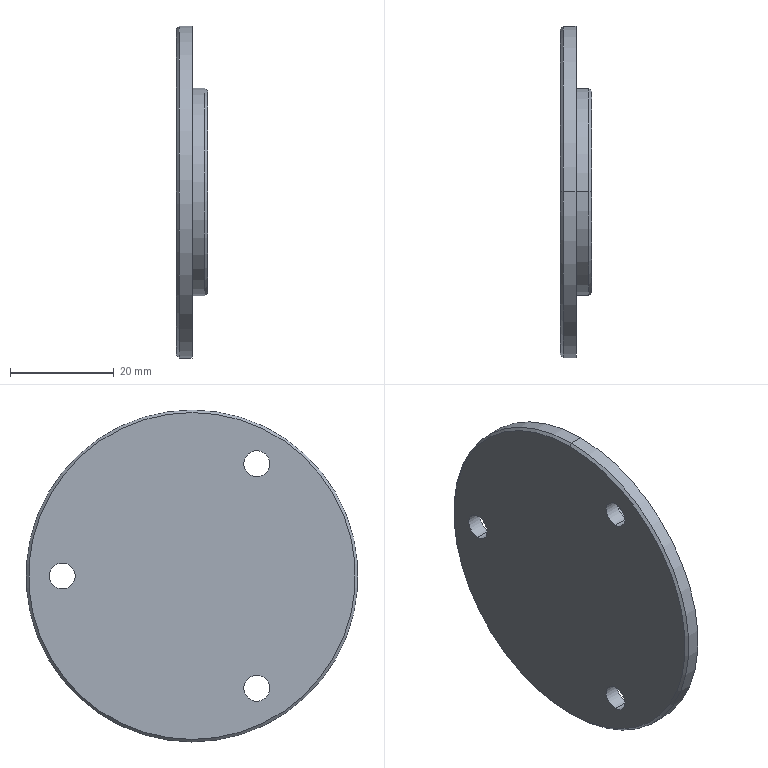Part | SolidWorks | features ICE 3, Chamfer 1, Extrusion 1 | 1 solid | 20 faces | box 6 x 64 x 64 mm | volume 11842 mm3 | cylinder 12 | cone 4 | plane 4 | commonest cylinder face diameters 5 x6 34 x2 40 x2 64 x2
STEP:
#1=CARTESIAN_POINT('',(0.,0.,31.5));
#2=VERTEX_POINT('',#1);
#3=CARTESIAN_POINT('',(0.,0.,-31.5));
#4=VERTEX_POINT('',#3);
#5=CARTESIAN_POINT('',(0.,0.,0.));
#6=DIRECTION('',(-1.,0.,0.));
#7=DIRECTION('',(0.,0.,-1.));
#8=AXIS2_PLACEMENT_3D('',#5,#6,#7);
#9=CIRCLE('',#8,31.5);
#10=EDGE_CURVE('',#2,#4,#9,.T.);
#11=ORIENTED_EDGE('',*,*,#10,.F.);
#12=CARTESIAN_POINT('',(0.5,0.,32.));
#13=VERTEX_POINT('',#12);
#14=CARTESIAN_POINT('',(0.5,0.,32.));
#15=DIRECTION('',(0.7071,0.,0.7071));
#16=VECTOR('',#15,1000.);
#17=LINE('',#14,#16);
#18=EDGE_CURVE('',#2,#13,#17,.T.);
#19=ORIENTED_EDGE('',*,*,#18,.T.);
#20=CARTESIAN_POINT('',(0.5,0.,-32.));
#21=VERTEX_POINT('',#20);
#22=CARTESIAN_POINT('',(0.5,0.,0.));
#23=DIRECTION('',(1.,0.,0.));
#24=DIRECTION('',(0.,0.,-1.));
#25=AXIS2_PLACEMENT_3D('',#22,#23,#24);
#26=CIRCLE('',#25,32.);
#27=EDGE_CURVE('',#21,#13,#26,.T.);
#28=ORIENTED_EDGE('',*,*,#27,.F.);
#29=CARTESIAN_POINT('',(0.5,0.,-32.));
#30=DIRECTION('',(0.7071,0.,-0.7071));
#31=VECTOR('',#30,1000.);
#32=LINE('',#29,#31);
#33=EDGE_CURVE('',#4,#21,#32,.T.);
#34=ORIENTED_EDGE('',*,*,#33,.F.);
#35=EDGE_LOOP('',(#11,#19,#28,#34));
#36=FACE_OUTER_BOUND('',#35,.T.);
#37=CARTESIAN_POINT('',(0.5,0.,0.));
#38=DIRECTION('',(1.,0.,0.));
#39=DIRECTION('',(0.,0.,-1.));
#40=AXIS2_PLACEMENT_3D('',#37,#38,#39);
#41=CONICAL_SURFACE('',#40,32.,0.7854);
#42=ADVANCED_FACE('',(#36),#41,.T.);
#43=CARTESIAN_POINT('',(6.,0.,-19.5));
#44=VERTEX_POINT('',#43);
#45=CARTESIAN_POINT('',(6.,0.,19.5));
#46=VERTEX_POINT('',#45);
#47=CARTESIAN_POINT('',(6.,0.,0.));
#48=DIRECTION('',(1.,0.,0.));
#49=DIRECTION('',(0.,0.,-1.));
#50=AXIS2_PLACEMENT_3D('',#47,#48,#49);
#51=CIRCLE('',#50,19.5);
#52=EDGE_CURVE('',#44,#46,#51,.T.);
#53=ORIENTED_EDGE('',*,*,#52,.F.);
#54=CARTESIAN_POINT('',(5.5,0.,-20.));
#55=VERTEX_POINT('',#54);
#56=CARTESIAN_POINT('',(6.,0.,-19.5));
#57=DIRECTION('',(-0.7071,0.,-0.7071));
#58=VECTOR('',#57,1000.);
#59=LINE('',#56,#58);
#60=EDGE_CURVE('',#44,#55,#59,.T.);
#61=ORIENTED_EDGE('',*,*,#60,.T.);
#62=CARTESIAN_POINT('',(5.5,0.,20.));
#63=VERTEX_POINT('',#62);
#64=CARTESIAN_POINT('',(5.5,0.,0.));
#65=DIRECTION('',(-1.,0.,0.));
#66=DIRECTION('',(0.,0.,-1.));
#67=AXIS2_PLACEMENT_3D('',#64,#65,#66);
#68=CIRCLE('',#67,20.);
#69=EDGE_CURVE('',#63,#55,#68,.T.);
#70=ORIENTED_EDGE('',*,*,#69,.F.);
#71=CARTESIAN_POINT('',(6.,0.,19.5));
#72=DIRECTION('',(-0.7071,0.,0.7071));
#73=VECTOR('',#72,1000.);
#74=LINE('',#71,#73);
#75=EDGE_CURVE('',#46,#63,#74,.T.);
#76=ORIENTED_EDGE('',*,*,#75,.F.);
#77=EDGE_LOOP('',(#53,#61,#70,#76));
#78=FACE_OUTER_BOUND('',#77,.T.);
#79=CARTESIAN_POINT('',(6.,0.,0.));
#80=DIRECTION('',(-1.,0.,0.));
#81=DIRECTION('',(0.,0.,1.));
#82=AXIS2_PLACEMENT_3D('',#79,#80,#81);
#83=CONICAL_SURFACE('',#82,19.5,0.7854);
#84=ADVANCED_FACE('',(#78),#83,.T.);
#85=CARTESIAN_POINT('',(3.,25.,2.5));
#86=VERTEX_POINT('',#85);
#87=CARTESIAN_POINT('',(3.,25.,-2.5));
#88=VERTEX_POINT('',#87);
#89=CARTESIAN_POINT('',(3.,25.,0.));
#90=DIRECTION('',(1.,0.,0.));
#91=DIRECTION('',(0.,0.,-1.));
#92=AXIS2_PLACEMENT_3D('',#89,#90,#91);
#93=CIRCLE('',#92,2.5);
#94=EDGE_CURVE('',#86,#88,#93,.T.);
#95=ORIENTED_EDGE('',*,*,#94,.T.);
#96=CARTESIAN_POINT('',(0.,25.,-2.5));
#97=VERTEX_POINT('',#96);
#98=CARTESIAN_POINT('',(36.5,25.,-2.5));
#99=DIRECTION('',(-1.,0.,0.));
#100=VECTOR('',#99,1000.);
#101=LINE('',#98,#100);
#102=EDGE_CURVE('',#88,#97,#101,.T.);
#103=ORIENTED_EDGE('',*,*,#102,.T.);
#104=CARTESIAN_POINT('',(0.,25.,2.5));
#105=VERTEX_POINT('',#104);
#106=CARTESIAN_POINT('',(0.,25.,0.));
#107=DIRECTION('',(-1.,0.,0.));
#108=DIRECTION('',(0.,0.,1.));
#109=AXIS2_PLACEMENT_3D('',#106,#107,#108);
#110=CIRCLE('',#109,2.5);
#111=EDGE_CURVE('',#97,#105,#110,.T.);
#112=ORIENTED_EDGE('',*,*,#111,.T.);
#113=CARTESIAN_POINT('',(36.5,25.,2.5));
#114=DIRECTION('',(-1.,0.,0.));
#115=VECTOR('',#114,1000.);
#116=LINE('',#113,#115);
#117=EDGE_CURVE('',#86,#105,#116,.T.);
#118=ORIENTED_EDGE('',*,*,#117,.F.);
#119=EDGE_LOOP('',(#95,#103,#112,#118));
#120=FACE_OUTER_BOUND('',#119,.T.);
#121=CARTESIAN_POINT('',(36.5,25.,0.));
#122=DIRECTION('',(-1.,0.,0.));
#123=DIRECTION('',(0.,0.,1.));
#124=AXIS2_PLACEMENT_3D('',#121,#122,#123);
#125=CYLINDRICAL_SURFACE('',#124,2.5);
#126=ADVANCED_FACE('',(#120),#125,.F.);
#127=CARTESIAN_POINT('',(3.,-12.5,24.151));
#128=VERTEX_POINT('',#127);
#129=CARTESIAN_POINT('',(3.,-12.5,19.151));
#130=VERTEX_POINT('',#129);
#131=CARTESIAN_POINT('',(3.,-12.5,21.651));
#132=DIRECTION('',(1.,0.,0.));
#133=DIRECTION('',(0.,0.,-1.));
#134=AXIS2_PLACEMENT_3D('',#131,#132,#133);
#135=CIRCLE('',#134,2.5);
#136=EDGE_CURVE('',#128,#130,#135,.T.);
#137=ORIENTED_EDGE('',*,*,#136,.T.);
#138=CARTESIAN_POINT('',(0.,-12.5,19.151));
#139=VERTEX_POINT('',#138);
#140=CARTESIAN_POINT('',(36.5,-12.5,19.151));
#141=DIRECTION('',(-1.,0.,0.));
#142=VECTOR('',#141,1000.);
#143=LINE('',#140,#142);
#144=EDGE_CURVE('',#130,#139,#143,.T.);
#145=ORIENTED_EDGE('',*,*,#144,.T.);
#146=CARTESIAN_POINT('',(0.,-12.5,24.151));
#147=VERTEX_POINT('',#146);
#148=CARTESIAN_POINT('',(0.,-12.5,21.651));
#149=DIRECTION('',(-1.,0.,0.));
#150=DIRECTION('',(0.,0.,1.));
#151=AXIS2_PLACEMENT_3D('',#148,#149,#150);
#152=CIRCLE('',#151,2.5);
#153=EDGE_CURVE('',#139,#147,#152,.T.);
#154=ORIENTED_EDGE('',*,*,#153,.T.);
#155=CARTESIAN_POINT('',(36.5,-12.5,24.151));
#156=DIRECTION('',(-1.,0.,0.));
#157=VECTOR('',#156,1000.);
#158=LINE('',#155,#157);
#159=EDGE_CURVE('',#128,#147,#158,.T.);
#160=ORIENTED_EDGE('',*,*,#159,.F.);
#161=EDGE_LOOP('',(#137,#145,#154,#160));
#162=FACE_OUTER_BOUND('',#161,.T.);
#163=CARTESIAN_POINT('',(36.5,-12.5,21.651));
#164=DIRECTION('',(-1.,0.,0.));
#165=DIRECTION('',(0.,0.,1.));
#166=AXIS2_PLACEMENT_3D('',#163,#164,#165);
#167=CYLINDRICAL_SURFACE('',#166,2.5);
#168=ADVANCED_FACE('',(#162),#167,.F.);
#169=CARTESIAN_POINT('',(3.,-12.5,-19.151));
#170=VERTEX_POINT('',#169);
#171=CARTESIAN_POINT('',(3.,-12.5,-24.151));
#172=VERTEX_POINT('',#171);
#173=CARTESIAN_POINT('',(3.,-12.5,-21.651));
#174=DIRECTION('',(1.,0.,0.));
#175=DIRECTION('',(0.,0.,-1.));
#176=AXIS2_PLACEMENT_3D('',#173,#174,#175);
#177=CIRCLE('',#176,2.5);
#178=EDGE_CURVE('',#170,#172,#177,.T.);
#179=ORIENTED_EDGE('',*,*,#178,.T.);
#180=CARTESIAN_POINT('',(0.,-12.5,-24.151));
#181=VERTEX_POINT('',#180);
#182=CARTESIAN_POINT('',(36.5,-12.5,-24.151));
#183=DIRECTION('',(-1.,0.,0.));
#184=VECTOR('',#183,1000.);
#185=LINE('',#182,#184);
#186=EDGE_CURVE('',#172,#181,#185,.T.);
#187=ORIENTED_EDGE('',*,*,#186,.T.);
#188=CARTESIAN_POINT('',(0.,-12.5,-19.151));
#189=VERTEX_POINT('',#188);
#190=CARTESIAN_POINT('',(0.,-12.5,-21.651));
#191=DIRECTION('',(-1.,0.,0.));
#192=DIRECTION('',(0.,0.,1.));
#193=AXIS2_PLACEMENT_3D('',#190,#191,#192);
#194=CIRCLE('',#193,2.5);
#195=EDGE_CURVE('',#181,#189,#194,.T.);
#196=ORIENTED_EDGE('',*,*,#195,.T.);
#197=CARTESIAN_POINT('',(36.5,-12.5,-19.151));
#198=DIRECTION('',(-1.,0.,0.));
#199=VECTOR('',#198,1000.);
#200=LINE('',#197,#199);
#201=EDGE_CURVE('',#170,#189,#200,.T.);
#202=ORIENTED_EDGE('',*,*,#201,.F.);
#203=EDGE_LOOP('',(#179,#187,#196,#202));
#204=FACE_OUTER_BOUND('',#203,.T.);
#205=CARTESIAN_POINT('',(36.5,-12.5,-21.651));
#206=DIRECTION('',(-1.,0.,0.));
#207=DIRECTION('',(0.,0.,1.));
#208=AXIS2_PLACEMENT_3D('',#205,#206,#207);
#209=CYLINDRICAL_SURFACE('',#208,2.5);
#210=ADVANCED_FACE('',(#204),#209,.F.);
#211=CARTESIAN_POINT('',(4.5,0.,17.));
#212=VERTEX_POINT('',#211);
#213=CARTESIAN_POINT('',(4.5,0.,-17.));
#214=VERTEX_POINT('',#213);
#215=CARTESIAN_POINT('',(4.5,0.,0.));
#216=DIRECTION('',(1.,0.,0.));
#217=DIRECTION('',(0.,0.,-1.));
#218=AXIS2_PLACEMENT_3D('',#215,#216,#217);
#219=CIRCLE('',#218,17.);
#220=EDGE_CURVE('',#212,#214,#219,.T.);
#221=ORIENTED_EDGE('',*,*,#220,.F.);
#222=CARTESIAN_POINT('',(6.,0.,17.));
#223=VERTEX_POINT('',#222);
#224=CARTESIAN_POINT('',(4.5,0.,17.));
#225=DIRECTION('',(1.,0.,0.));
#226=VECTOR('',#225,1000.);
#227=LINE('',#224,#226);
#228=EDGE_CURVE('',#212,#223,#227,.T.);
#229=ORIENTED_EDGE('',*,*,#228,.T.);
#230=CARTESIAN_POINT('',(6.,0.,-17.));
#231=VERTEX_POINT('',#230);
#232=CARTESIAN_POINT('',(6.,0.,0.));
#233=DIRECTION('',(1.,0.,0.));
#234=DIRECTION('',(0.,0.,-1.));
#235=AXIS2_PLACEMENT_3D('',#232,#233,#234);
#236=CIRCLE('',#235,17.);
#237=EDGE_CURVE('',#223,#231,#236,.T.);
#238=ORIENTED_EDGE('',*,*,#237,.T.);
#239=CARTESIAN_POINT('',(4.5,0.,-17.));
#240=DIRECTION('',(1.,0.,0.));
#241=VECTOR('',#240,1000.);
#242=LINE('',#239,#241);
#243=EDGE_CURVE('',#214,#231,#242,.T.);
#244=ORIENTED_EDGE('',*,*,#243,.F.);
#245=EDGE_LOOP('',(#221,#229,#238,#244));
#246=FACE_OUTER_BOUND('',#245,.T.);
#247=CARTESIAN_POINT('',(4.5,0.,0.));
#248=DIRECTION('',(1.,0.,0.));
#249=DIRECTION('',(0.,0.,-1.));
#250=AXIS2_PLACEMENT_3D('',#247,#248,#249);
#251=CYLINDRICAL_SURFACE('',#250,17.);
#252=ADVANCED_FACE('',(#246),#251,.F.);
#253=ORIENTED_EDGE('',*,*,#69,.T.);
#254=CARTESIAN_POINT('',(3.,0.,-20.));
#255=VERTEX_POINT('',#254);
#256=CARTESIAN_POINT('',(6.,0.,-20.));
#257=DIRECTION('',(-1.,0.,0.));
#258=VECTOR('',#257,1000.);
#259=LINE('',#256,#258);
#260=EDGE_CURVE('',#55,#255,#259,.T.);
#261=ORIENTED_EDGE('',*,*,#260,.T.);
#262=CARTESIAN_POINT('',(3.,0.,20.));
#263=VERTEX_POINT('',#262);
#264=CARTESIAN_POINT('',(3.,0.,0.));
#265=DIRECTION('',(1.,0.,0.));
#266=DIRECTION('',(0.,0.,-1.));
#267=AXIS2_PLACEMENT_3D('',#264,#265,#266);
#268=CIRCLE('',#267,20.);
#269=EDGE_CURVE('',#255,#263,#268,.T.);
#270=ORIENTED_EDGE('',*,*,#269,.T.);
#271=CARTESIAN_POINT('',(6.,0.,20.));
#272=DIRECTION('',(-1.,0.,0.));
#273=VECTOR('',#272,1000.);
#274=LINE('',#271,#273);
#275=EDGE_CURVE('',#63,#263,#274,.T.);
#276=ORIENTED_EDGE('',*,*,#275,.F.);
#277=EDGE_LOOP('',(#253,#261,#270,#276));
#278=FACE_OUTER_BOUND('',#277,.T.);
#279=CARTESIAN_POINT('',(6.,0.,0.));
#280=DIRECTION('',(-1.,0.,0.));
#281=DIRECTION('',(0.,0.,1.));
#282=AXIS2_PLACEMENT_3D('',#279,#280,#281);
#283=CYLINDRICAL_SURFACE('',#282,20.);
#284=ADVANCED_FACE('',(#278),#283,.T.);
#285=CARTESIAN_POINT('',(3.,0.,-32.));
#286=VERTEX_POINT('',#285);
#287=CARTESIAN_POINT('',(3.,0.,32.));
#288=VERTEX_POINT('',#287);
#289=CARTESIAN_POINT('',(3.,0.,0.));
#290=DIRECTION('',(1.,0.,0.));
#291=DIRECTION('',(0.,0.,-1.));
#292=AXIS2_PLACEMENT_3D('',#289,#290,#291);
#293=CIRCLE('',#292,32.);
#294=EDGE_CURVE('',#286,#288,#293,.T.);
#295=ORIENTED_EDGE('',*,*,#294,.F.);
#296=CARTESIAN_POINT('',(3.,0.,-32.));
#297=DIRECTION('',(-1.,0.,0.));
#298=VECTOR('',#297,1000.);
#299=LINE('',#296,#298);
#300=EDGE_CURVE('',#286,#21,#299,.T.);
#301=ORIENTED_EDGE('',*,*,#300,.T.);
#302=ORIENTED_EDGE('',*,*,#27,.T.);
#303=CARTESIAN_POINT('',(3.,0.,32.));
#304=DIRECTION('',(-1.,0.,0.));
#305=VECTOR('',#304,1000.);
#306=LINE('',#303,#305);
#307=EDGE_CURVE('',#288,#13,#306,.T.);
#308=ORIENTED_EDGE('',*,*,#307,.F.);
#309=EDGE_LOOP('',(#295,#301,#302,#308));
#310=FACE_OUTER_BOUND('',#309,.T.);
#311=CARTESIAN_POINT('',(3.,0.,0.));
#312=DIRECTION('',(-1.,0.,0.));
#313=DIRECTION('',(0.,0.,1.));
#314=AXIS2_PLACEMENT_3D('',#311,#312,#313);
#315=CYLINDRICAL_SURFACE('',#314,32.);
#316=ADVANCED_FACE('',(#310),#315,.T.);
#317=ORIENTED_EDGE('',*,*,#300,.F.);
#318=CARTESIAN_POINT('',(3.,0.,0.));
#319=DIRECTION('',(1.,0.,0.));
#320=DIRECTION('',(0.,0.,-1.));
#321=AXIS2_PLACEMENT_3D('',#318,#319,#320);
#322=CIRCLE('',#321,32.);
#323=EDGE_CURVE('',#288,#286,#322,.T.);
#324=ORIENTED_EDGE('',*,*,#323,.F.);
#325=ORIENTED_EDGE('',*,*,#307,.T.);
#326=CARTESIAN_POINT('',(0.5,0.,0.));
#327=DIRECTION('',(1.,0.,0.));
#328=DIRECTION('',(0.,0.,-1.));
#329=AXIS2_PLACEMENT_3D('',#326,#327,#328);
#330=CIRCLE('',#329,32.);
#331=EDGE_CURVE('',#13,#21,#330,.T.);
#332=ORIENTED_EDGE('',*,*,#331,.T.);
#333=EDGE_LOOP('',(#317,#324,#325,#332));
#334=FACE_OUTER_BOUND('',#333,.T.);
#335=CARTESIAN_POINT('',(3.,0.,0.));
#336=DIRECTION('',(-1.,0.,0.));
#337=DIRECTION('',(0.,0.,1.));
#338=AXIS2_PLACEMENT_3D('',#335,#336,#337);
#339=CYLINDRICAL_SURFACE('',#338,32.);
#340=ADVANCED_FACE('',(#334),#339,.T.);
#341=ORIENTED_EDGE('',*,*,#94,.F.);
#342=CARTESIAN_POINT('',(3.,25.,0.));
#343=DIRECTION('',(1.,0.,0.));
#344=DIRECTION('',(0.,0.,-1.));
#345=AXIS2_PLACEMENT_3D('',#342,#343,#344);
#346=CIRCLE('',#345,2.5);
#347=EDGE_CURVE('',#88,#86,#346,.T.);
#348=ORIENTED_EDGE('',*,*,#347,.F.);
#349=EDGE_LOOP('',(#341,#348));
#350=FACE_BOUND('',#349,.T.);
#351=ORIENTED_EDGE('',*,*,#136,.F.);
#352=CARTESIAN_POINT('',(3.,-12.5,21.651));
#353=DIRECTION('',(1.,0.,0.));
#354=DIRECTION('',(0.,0.,-1.));
#355=AXIS2_PLACEMENT_3D('',#352,#353,#354);
#356=CIRCLE('',#355,2.5);
#357=EDGE_CURVE('',#130,#128,#356,.T.);
#358=ORIENTED_EDGE('',*,*,#357,.F.);
#359=EDGE_LOOP('',(#351,#358));
#360=FACE_BOUND('',#359,.T.);
#361=ORIENTED_EDGE('',*,*,#178,.F.);
#362=CARTESIAN_POINT('',(3.,-12.5,-21.651));
#363=DIRECTION('',(1.,0.,0.));
#364=DIRECTION('',(0.,0.,-1.));
#365=AXIS2_PLACEMENT_3D('',#362,#363,#364);
#366=CIRCLE('',#365,2.5);
#367=EDGE_CURVE('',#172,#170,#366,.T.);
#368=ORIENTED_EDGE('',*,*,#367,.F.);
#369=EDGE_LOOP('',(#361,#368));
#370=FACE_BOUND('',#369,.T.);
#371=CARTESIAN_POINT('',(3.,0.,0.));
#372=DIRECTION('',(1.,0.,0.));
#373=DIRECTION('',(0.,0.,-1.));
#374=AXIS2_PLACEMENT_3D('',#371,#372,#373);
#375=CIRCLE('',#374,20.);
#376=EDGE_CURVE('',#263,#255,#375,.T.);
#377=ORIENTED_EDGE('',*,*,#376,.F.);
#378=ORIENTED_EDGE('',*,*,#269,.F.);
#379=EDGE_LOOP('',(#377,#378));
#380=FACE_BOUND('',#379,.T.);
#381=ORIENTED_EDGE('',*,*,#323,.T.);
#382=ORIENTED_EDGE('',*,*,#294,.T.);
#383=EDGE_LOOP('',(#381,#382));
#384=FACE_OUTER_BOUND('',#383,.T.);
#385=CARTESIAN_POINT('',(3.,0.,0.));
#386=DIRECTION('',(1.,0.,0.));
#387=DIRECTION('',(0.,0.,-1.));
#388=AXIS2_PLACEMENT_3D('',#385,#386,#387);
#389=PLANE('',#388);
#390=ADVANCED_FACE('',(#350,#360,#370,#380,#384),#389,.T.);
#391=CARTESIAN_POINT('',(0.,0.,0.));
#392=DIRECTION('',(-1.,0.,0.));
#393=DIRECTION('',(0.,0.,-1.));
#394=AXIS2_PLACEMENT_3D('',#391,#392,#393);
#395=CIRCLE('',#394,31.5);
#396=EDGE_CURVE('',#4,#2,#395,.T.);
#397=ORIENTED_EDGE('',*,*,#396,.T.);
#398=ORIENTED_EDGE('',*,*,#10,.T.);
#399=EDGE_LOOP('',(#397,#398));
#400=FACE_OUTER_BOUND('',#399,.T.);
#401=CARTESIAN_POINT('',(0.,25.,0.));
#402=DIRECTION('',(-1.,0.,0.));
#403=DIRECTION('',(0.,0.,1.));
#404=AXIS2_PLACEMENT_3D('',#401,#402,#403);
#405=CIRCLE('',#404,2.5);
#406=EDGE_CURVE('',#105,#97,#405,.T.);
#407=ORIENTED_EDGE('',*,*,#406,.F.);
#408=ORIENTED_EDGE('',*,*,#111,.F.);
#409=EDGE_LOOP('',(#407,#408));
#410=FACE_BOUND('',#409,.T.);
#411=CARTESIAN_POINT('',(0.,-12.5,21.651));
#412=DIRECTION('',(-1.,0.,0.));
#413=DIRECTION('',(0.,0.,1.));
#414=AXIS2_PLACEMENT_3D('',#411,#412,#413);
#415=CIRCLE('',#414,2.5);
#416=EDGE_CURVE('',#147,#139,#415,.T.);
#417=ORIENTED_EDGE('',*,*,#416,.F.);
#418=ORIENTED_EDGE('',*,*,#153,.F.);
#419=EDGE_LOOP('',(#417,#418));
#420=FACE_BOUND('',#419,.T.);
#421=CARTESIAN_POINT('',(0.,-12.5,-21.651));
#422=DIRECTION('',(-1.,0.,0.));
#423=DIRECTION('',(0.,0.,1.));
#424=AXIS2_PLACEMENT_3D('',#421,#422,#423);
#425=CIRCLE('',#424,2.5);
#426=EDGE_CURVE('',#189,#181,#425,.T.);
#427=ORIENTED_EDGE('',*,*,#426,.F.);
#428=ORIENTED_EDGE('',*,*,#195,.F.);
#429=EDGE_LOOP('',(#427,#428));
#430=FACE_BOUND('',#429,.T.);
#431=CARTESIAN_POINT('',(0.,0.,0.));
#432=DIRECTION('',(1.,0.,0.));
#433=DIRECTION('',(0.,0.,-1.));
#434=AXIS2_PLACEMENT_3D('',#431,#432,#433);
#435=PLANE('',#434);
#436=ADVANCED_FACE('',(#400,#410,#420,#430),#435,.F.);
#437=ORIENTED_EDGE('',*,*,#260,.F.);
#438=CARTESIAN_POINT('',(5.5,0.,0.));
#439=DIRECTION('',(-1.,0.,0.));
#440=DIRECTION('',(0.,0.,-1.));
#441=AXIS2_PLACEMENT_3D('',#438,#439,#440);
#442=CIRCLE('',#441,20.);
#443=EDGE_CURVE('',#55,#63,#442,.T.);
#444=ORIENTED_EDGE('',*,*,#443,.T.);
#445=ORIENTED_EDGE('',*,*,#275,.T.);
#446=ORIENTED_EDGE('',*,*,#376,.T.);
#447=EDGE_LOOP('',(#437,#444,#445,#446));
#448=FACE_OUTER_BOUND('',#447,.T.);
#449=CARTESIAN_POINT('',(6.,0.,0.));
#450=DIRECTION('',(-1.,0.,0.));
#451=DIRECTION('',(0.,0.,1.));
#452=AXIS2_PLACEMENT_3D('',#449,#450,#451);
#453=CYLINDRICAL_SURFACE('',#452,20.);
#454=ADVANCED_FACE('',(#448),#453,.T.);
#455=CARTESIAN_POINT('',(6.,0.,0.));
#456=DIRECTION('',(1.,0.,0.));
#457=DIRECTION('',(0.,0.,-1.));
#458=AXIS2_PLACEMENT_3D('',#455,#456,#457);
#459=CIRCLE('',#458,19.5);
#460=EDGE_CURVE('',#46,#44,#459,.T.);
#461=ORIENTED_EDGE('',*,*,#460,.T.);
#462=ORIENTED_EDGE('',*,*,#52,.T.);
#463=EDGE_LOOP('',(#461,#462));
#464=FACE_OUTER_BOUND('',#463,.T.);
#465=CARTESIAN_POINT('',(6.,0.,0.));
#466=DIRECTION('',(1.,0.,0.));
#467=DIRECTION('',(0.,0.,-1.));
#468=AXIS2_PLACEMENT_3D('',#465,#466,#467);
#469=CIRCLE('',#468,17.);
#470=EDGE_CURVE('',#231,#223,#469,.T.);
#471=ORIENTED_EDGE('',*,*,#470,.F.);
#472=ORIENTED_EDGE('',*,*,#237,.F.);
#473=EDGE_LOOP('',(#471,#472));
#474=FACE_BOUND('',#473,.T.);
#475=CARTESIAN_POINT('',(6.,0.,0.));
#476=DIRECTION('',(1.,0.,0.));
#477=DIRECTION('',(0.,0.,-1.));
#478=AXIS2_PLACEMENT_3D('',#475,#476,#477);
#479=PLANE('',#478);
#480=ADVANCED_FACE('',(#464,#474),#479,.T.);
#481=ORIENTED_EDGE('',*,*,#228,.F.);
#482=CARTESIAN_POINT('',(4.5,0.,0.));
#483=DIRECTION('',(1.,0.,0.));
#484=DIRECTION('',(0.,0.,-1.));
#485=AXIS2_PLACEMENT_3D('',#482,#483,#484);
#486=CIRCLE('',#485,17.);
#487=EDGE_CURVE('',#214,#212,#486,.T.);
#488=ORIENTED_EDGE('',*,*,#487,.F.);
#489=ORIENTED_EDGE('',*,*,#243,.T.);
#490=ORIENTED_EDGE('',*,*,#470,.T.);
#491=EDGE_LOOP('',(#481,#488,#489,#490));
#492=FACE_OUTER_BOUND('',#491,.T.);
#493=CARTESIAN_POINT('',(4.5,0.,0.));
#494=DIRECTION('',(1.,0.,0.));
#495=DIRECTION('',(0.,0.,-1.));
#496=AXIS2_PLACEMENT_3D('',#493,#494,#495);
#497=CYLINDRICAL_SURFACE('',#496,17.);
#498=ADVANCED_FACE('',(#492),#497,.F.);
#499=ORIENTED_EDGE('',*,*,#487,.T.);
#500=ORIENTED_EDGE('',*,*,#220,.T.);
#501=EDGE_LOOP('',(#499,#500));
#502=FACE_OUTER_BOUND('',#501,.T.);
#503=CARTESIAN_POINT('',(4.5,0.,0.));
#504=DIRECTION('',(1.,0.,0.));
#505=DIRECTION('',(0.,0.,-1.));
#506=AXIS2_PLACEMENT_3D('',#503,#504,#505);
#507=PLANE('',#506);
#508=ADVANCED_FACE('',(#502),#507,.T.);
#509=ORIENTED_EDGE('',*,*,#186,.F.);
#510=ORIENTED_EDGE('',*,*,#367,.T.);
#511=ORIENTED_EDGE('',*,*,#201,.T.);
#512=ORIENTED_EDGE('',*,*,#426,.T.);
#513=EDGE_LOOP('',(#509,#510,#511,#512));
#514=FACE_OUTER_BOUND('',#513,.T.);
#515=CARTESIAN_POINT('',(36.5,-12.5,-21.651));
#516=DIRECTION('',(-1.,0.,0.));
#517=DIRECTION('',(0.,0.,1.));
#518=AXIS2_PLACEMENT_3D('',#515,#516,#517);
#519=CYLINDRICAL_SURFACE('',#518,2.5);
#520=ADVANCED_FACE('',(#514),#519,.F.);
#521=ORIENTED_EDGE('',*,*,#144,.F.);
#522=ORIENTED_EDGE('',*,*,#357,.T.);
#523=ORIENTED_EDGE('',*,*,#159,.T.);
#524=ORIENTED_EDGE('',*,*,#416,.T.);
#525=EDGE_LOOP('',(#521,#522,#523,#524));
#526=FACE_OUTER_BOUND('',#525,.T.);
#527=CARTESIAN_POINT('',(36.5,-12.5,21.651));
#528=DIRECTION('',(-1.,0.,0.));
#529=DIRECTION('',(0.,0.,1.));
#530=AXIS2_PLACEMENT_3D('',#527,#528,#529);
#531=CYLINDRICAL_SURFACE('',#530,2.5);
#532=ADVANCED_FACE('',(#526),#531,.F.);
#533=ORIENTED_EDGE('',*,*,#102,.F.);
#534=ORIENTED_EDGE('',*,*,#347,.T.);
#535=ORIENTED_EDGE('',*,*,#117,.T.);
#536=ORIENTED_EDGE('',*,*,#406,.T.);
#537=EDGE_LOOP('',(#533,#534,#535,#536));
#538=FACE_OUTER_BOUND('',#537,.T.);
#539=CARTESIAN_POINT('',(36.5,25.,0.));
#540=DIRECTION('',(-1.,0.,0.));
#541=DIRECTION('',(0.,0.,1.));
#542=AXIS2_PLACEMENT_3D('',#539,#540,#541);
#543=CYLINDRICAL_SURFACE('',#542,2.5);
#544=ADVANCED_FACE('',(#538),#543,.F.);
#545=ORIENTED_EDGE('',*,*,#60,.F.);
#546=ORIENTED_EDGE('',*,*,#460,.F.);
#547=ORIENTED_EDGE('',*,*,#75,.T.);
#548=ORIENTED_EDGE('',*,*,#443,.F.);
#549=EDGE_LOOP('',(#545,#546,#547,#548));
#550=FACE_OUTER_BOUND('',#549,.T.);
#551=CARTESIAN_POINT('',(6.,0.,0.));
#552=DIRECTION('',(-1.,0.,0.));
#553=DIRECTION('',(0.,0.,1.));
#554=AXIS2_PLACEMENT_3D('',#551,#552,#553);
#555=CONICAL_SURFACE('',#554,19.5,0.7854);
#556=ADVANCED_FACE('',(#550),#555,.T.);
#557=ORIENTED_EDGE('',*,*,#18,.F.);
#558=ORIENTED_EDGE('',*,*,#396,.F.);
#559=ORIENTED_EDGE('',*,*,#33,.T.);
#560=ORIENTED_EDGE('',*,*,#331,.F.);
#561=EDGE_LOOP('',(#557,#558,#559,#560));
#562=FACE_OUTER_BOUND('',#561,.T.);
#563=CARTESIAN_POINT('',(0.5,0.,0.));
#564=DIRECTION('',(1.,0.,0.));
#565=DIRECTION('',(0.,0.,-1.));
#566=AXIS2_PLACEMENT_3D('',#563,#564,#565);
#567=CONICAL_SURFACE('',#566,32.,0.7854);
#568=ADVANCED_FACE('',(#562),#567,.T.);
#569=CLOSED_SHELL('',(#42,#84,#126,#168,#210,#252,#284,#316,#340,#390,#436,#454,#480,#498,#508,#520,#532,#544,#556,#568));
#570=MANIFOLD_SOLID_BREP('',#569);
#571=CARTESIAN_POINT('',(0.,0.,0.));
#572=DIRECTION('',(0.,0.,1.));
#573=DIRECTION('',(1.,0.,0.));
#574=AXIS2_PLACEMENT_3D('',#571,#572,#573);
#575=(LENGTH_UNIT()NAMED_UNIT(*)SI_UNIT(.MILLI.,.METRE.));
#576=UNCERTAINTY_MEASURE_WITH_UNIT(LENGTH_MEASURE(0.00001),#575,'','');
#577=(NAMED_UNIT(*)PLANE_ANGLE_UNIT()SI_UNIT($,.RADIAN.));
#578=(NAMED_UNIT(*)SI_UNIT($,.STERADIAN.)SOLID_ANGLE_UNIT());
#579=(GEOMETRIC_REPRESENTATION_CONTEXT(3)GLOBAL_UNCERTAINTY_ASSIGNED_CONTEXT((#576))GLOBAL_UNIT_ASSIGNED_CONTEXT((#575,#577,#578))REPRESENTATION_CONTEXT('',''));
#580=ADVANCED_BREP_SHAPE_REPRESENTATION('',(#570,#574),#579);